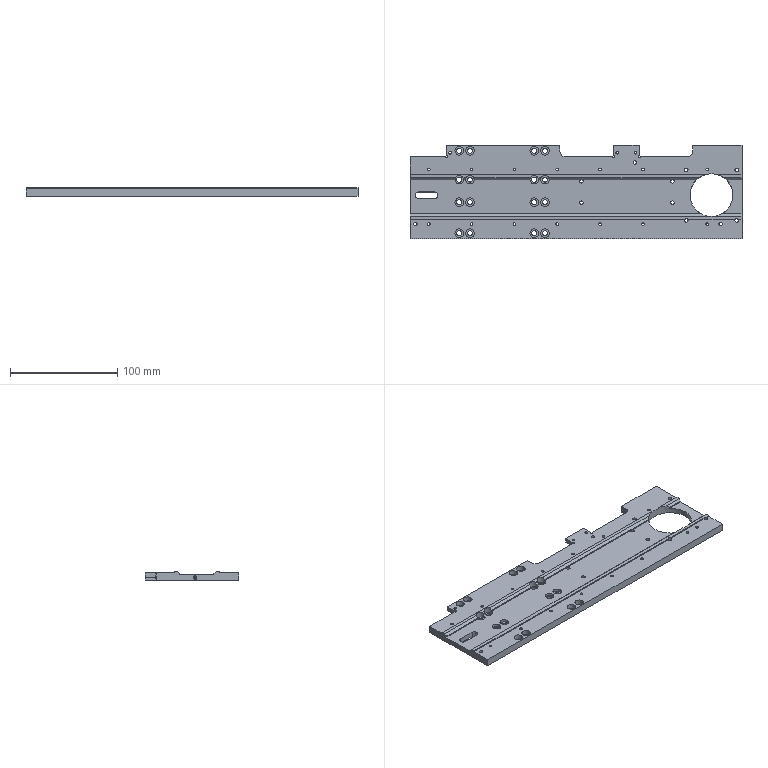Part | STEP file | 02-13Y轴底Plate | 1 solid | 223 faces | box 310 x 87 x 8 mm | volume 147659 mm3 | cylinder 143 | plane 72 | cone 8 | commonest cylinder face diameters 2.5 x36 8 x32 3.3 x28 4.5 x16 4.8 x16 2 x8